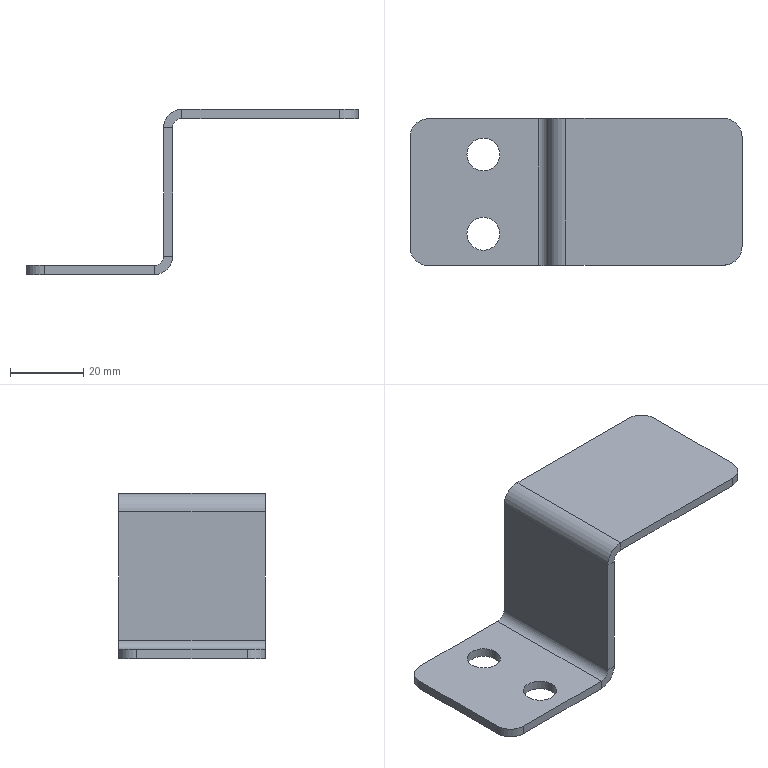Part | STEP file | 1 solid | 30 faces | box 90.5 x 40 x 45 mm | volume 12606 mm3 | plane 18 | cylinder 12 | commonest cylinder face diameters 10 x6 9 x4 5 x2